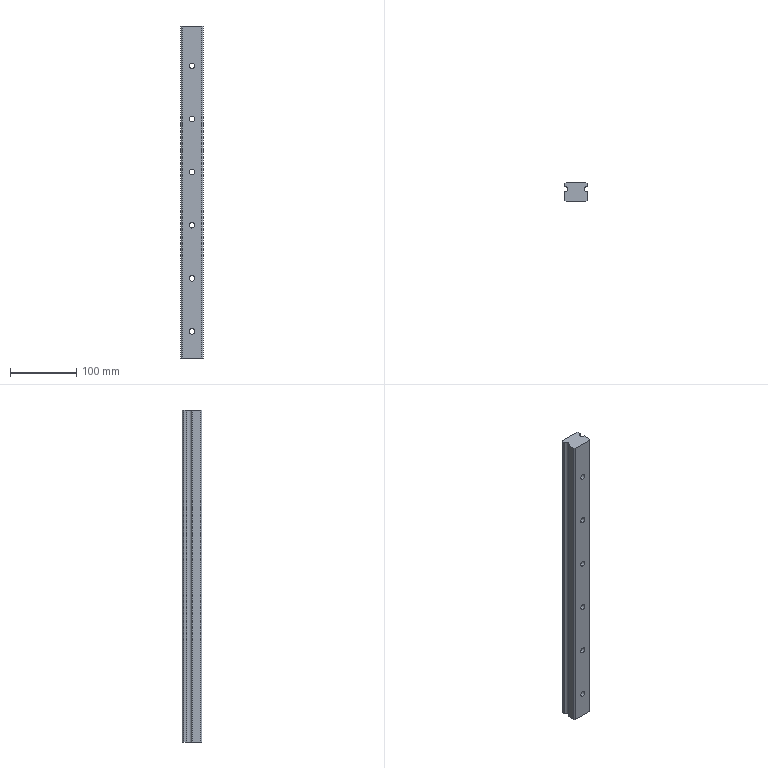Part | Creo | features CUT 7, CURVE 3, DATUM PLANE 3, COORDINATE SYSTEM 1, PATTERN 1, PROTRUSION 1 | 1 solid | 44 faces | box 33.99 x 29 x 500 mm | volume 443618 mm3 | cylinder 26 | plane 18 | commonest cylinder face diameters 8.5 x12 14 x12 8.76 x2
STEP:
#1=CARTESIAN_POINT('',(0.,0.,0.));
#2=DIRECTION('',(0.,0.,1.));
#3=DIRECTION('',(1.,0.,0.));
#4=AXIS2_PLACEMENT_3D('',#1,#2,#3);
#5=CARTESIAN_POINT('',(-14.995,0.,-250.));
#6=VERTEX_POINT('',#5);
#7=CARTESIAN_POINT('',(15.005,0.,-250.));
#8=VERTEX_POINT('',#7);
#9=CARTESIAN_POINT('',(-14.995,0.,-250.));
#10=DIRECTION('',(1.,0.,0.));
#11=VECTOR('',#10,30.);
#12=LINE('',#9,#11);
#13=EDGE_CURVE('',#6,#8,#12,.T.);
#14=ORIENTED_EDGE('',*,*,#13,.T.);
#15=CARTESIAN_POINT('',(17.,1.995,-250.));
#16=VERTEX_POINT('',#15);
#17=CARTESIAN_POINT('',(15.005,0.,-250.));
#18=DIRECTION('',(0.7071,0.7071,0.));
#19=VECTOR('',#18,2.821);
#20=LINE('',#17,#19);
#21=EDGE_CURVE('',#8,#16,#20,.T.);
#22=ORIENTED_EDGE('',*,*,#21,.T.);
#23=CARTESIAN_POINT('',(17.,14.215,-250.));
#24=VERTEX_POINT('',#23);
#25=CARTESIAN_POINT('',(17.,1.995,-250.));
#26=DIRECTION('',(0.,1.,0.));
#27=VECTOR('',#26,12.22);
#28=LINE('',#25,#27);
#29=EDGE_CURVE('',#16,#24,#28,.T.);
#30=ORIENTED_EDGE('',*,*,#29,.T.);
#31=CARTESIAN_POINT('',(17.,22.975,-250.));
#32=VERTEX_POINT('',#31);
#33=CARTESIAN_POINT('',(17.,18.595,-250.));
#34=DIRECTION('',(0.,0.,-1.));
#35=DIRECTION('',(0.,-1.,0.));
#36=AXIS2_PLACEMENT_3D('',#33,#34,#35);
#37=CIRCLE('',#36,4.38);
#38=EDGE_CURVE('',#24,#32,#37,.T.);
#39=ORIENTED_EDGE('',*,*,#38,.T.);
#40=CARTESIAN_POINT('',(17.,27.005,-250.));
#41=VERTEX_POINT('',#40);
#42=CARTESIAN_POINT('',(17.,22.975,-250.));
#43=DIRECTION('',(0.,1.,0.));
#44=VECTOR('',#43,4.03);
#45=LINE('',#42,#44);
#46=EDGE_CURVE('',#32,#41,#45,.T.);
#47=ORIENTED_EDGE('',*,*,#46,.T.);
#48=CARTESIAN_POINT('',(15.005,29.,-250.));
#49=VERTEX_POINT('',#48);
#50=CARTESIAN_POINT('',(17.,27.005,-250.));
#51=DIRECTION('',(-0.7071,0.7071,0.));
#52=VECTOR('',#51,2.821);
#53=LINE('',#50,#52);
#54=EDGE_CURVE('',#41,#49,#53,.T.);
#55=ORIENTED_EDGE('',*,*,#54,.T.);
#56=CARTESIAN_POINT('',(-14.995,29.,-250.));
#57=VERTEX_POINT('',#56);
#58=CARTESIAN_POINT('',(15.005,29.,-250.));
#59=DIRECTION('',(-1.,0.,0.));
#60=VECTOR('',#59,30.);
#61=LINE('',#58,#60);
#62=EDGE_CURVE('',#49,#57,#61,.T.);
#63=ORIENTED_EDGE('',*,*,#62,.T.);
#64=CARTESIAN_POINT('',(-16.99,27.005,-250.));
#65=VERTEX_POINT('',#64);
#66=CARTESIAN_POINT('',(-14.995,29.,-250.));
#67=DIRECTION('',(-0.7071,-0.7071,0.));
#68=VECTOR('',#67,2.821);
#69=LINE('',#66,#68);
#70=EDGE_CURVE('',#57,#65,#69,.T.);
#71=ORIENTED_EDGE('',*,*,#70,.T.);
#72=CARTESIAN_POINT('',(-16.99,22.975,-250.));
#73=VERTEX_POINT('',#72);
#74=CARTESIAN_POINT('',(-16.99,27.005,-250.));
#75=DIRECTION('',(0.,-1.,0.));
#76=VECTOR('',#75,4.03);
#77=LINE('',#74,#76);
#78=EDGE_CURVE('',#65,#73,#77,.T.);
#79=ORIENTED_EDGE('',*,*,#78,.T.);
#80=CARTESIAN_POINT('',(-16.99,14.215,-250.));
#81=VERTEX_POINT('',#80);
#82=CARTESIAN_POINT('',(-16.99,18.595,-250.));
#83=DIRECTION('',(0.,0.,-1.));
#84=DIRECTION('',(0.,1.,0.));
#85=AXIS2_PLACEMENT_3D('',#82,#83,#84);
#86=CIRCLE('',#85,4.38);
#87=EDGE_CURVE('',#73,#81,#86,.T.);
#88=ORIENTED_EDGE('',*,*,#87,.T.);
#89=CARTESIAN_POINT('',(-16.99,1.995,-250.));
#90=VERTEX_POINT('',#89);
#91=CARTESIAN_POINT('',(-16.99,14.215,-250.));
#92=DIRECTION('',(0.,-1.,0.));
#93=VECTOR('',#92,12.22);
#94=LINE('',#91,#93);
#95=EDGE_CURVE('',#81,#90,#94,.T.);
#96=ORIENTED_EDGE('',*,*,#95,.T.);
#97=CARTESIAN_POINT('',(-16.99,1.995,-250.));
#98=DIRECTION('',(0.7071,-0.7071,0.));
#99=VECTOR('',#98,2.821);
#100=LINE('',#97,#99);
#101=EDGE_CURVE('',#90,#6,#100,.T.);
#102=ORIENTED_EDGE('',*,*,#101,.T.);
#103=EDGE_LOOP('',(#14,#22,#30,#39,#47,#55,#63,#71,#79,#88,#96,#102));
#104=FACE_OUTER_BOUND('',#103,.F.);
#105=CARTESIAN_POINT('',(0.,0.,-250.));
#106=DIRECTION('',(0.,0.,1.));
#107=DIRECTION('',(1.,0.,0.));
#108=AXIS2_PLACEMENT_3D('',#105,#106,#107);
#109=PLANE('',#108);
#110=ADVANCED_FACE('',(#104),#109,.F.);
#111=ORIENTED_EDGE('',*,*,#13,.F.);
#112=CARTESIAN_POINT('',(-14.995,0.,250.));
#113=VERTEX_POINT('',#112);
#114=CARTESIAN_POINT('',(-14.995,0.,-250.));
#115=DIRECTION('',(0.,0.,1.));
#116=VECTOR('',#115,500.);
#117=LINE('',#114,#116);
#118=EDGE_CURVE('',#6,#113,#117,.T.);
#119=ORIENTED_EDGE('',*,*,#118,.T.);
#120=CARTESIAN_POINT('',(15.005,0.,250.));
#121=VERTEX_POINT('',#120);
#122=CARTESIAN_POINT('',(-14.995,0.,250.));
#123=DIRECTION('',(1.,0.,0.));
#124=VECTOR('',#123,30.);
#125=LINE('',#122,#124);
#126=EDGE_CURVE('',#113,#121,#125,.T.);
#127=ORIENTED_EDGE('',*,*,#126,.T.);
#128=CARTESIAN_POINT('',(15.005,0.,-250.));
#129=DIRECTION('',(0.,0.,1.));
#130=VECTOR('',#129,500.);
#131=LINE('',#128,#130);
#132=EDGE_CURVE('',#8,#121,#131,.T.);
#133=ORIENTED_EDGE('',*,*,#132,.F.);
#134=EDGE_LOOP('',(#111,#119,#127,#133));
#135=FACE_OUTER_BOUND('',#134,.F.);
#136=CARTESIAN_POINT('',(0.,0.,-214.25));
#137=VERTEX_POINT('',#136);
#138=CARTESIAN_POINT('',(0.,0.,-205.75));
#139=VERTEX_POINT('',#138);
#140=CARTESIAN_POINT('',(0.,0.,-210.));
#141=DIRECTION('',(0.,1.,0.));
#142=DIRECTION('',(0.,0.,-1.));
#143=AXIS2_PLACEMENT_3D('',#140,#141,#142);
#144=CIRCLE('',#143,4.25);
#145=EDGE_CURVE('',#137,#139,#144,.T.);
#146=ORIENTED_EDGE('',*,*,#145,.F.);
#147=CARTESIAN_POINT('',(0.,0.,-210.));
#148=DIRECTION('',(0.,1.,0.));
#149=DIRECTION('',(0.,0.,1.));
#150=AXIS2_PLACEMENT_3D('',#147,#148,#149);
#151=CIRCLE('',#150,4.25);
#152=EDGE_CURVE('',#139,#137,#151,.T.);
#153=ORIENTED_EDGE('',*,*,#152,.F.);
#154=EDGE_LOOP('',(#146,#153));
#155=FACE_BOUND('',#154,.F.);
#156=CARTESIAN_POINT('',(0.,0.,-134.25));
#157=VERTEX_POINT('',#156);
#158=CARTESIAN_POINT('',(0.,0.,-125.75));
#159=VERTEX_POINT('',#158);
#160=CARTESIAN_POINT('',(0.,0.,-130.));
#161=DIRECTION('',(0.,1.,0.));
#162=DIRECTION('',(0.,0.,-1.));
#163=AXIS2_PLACEMENT_3D('',#160,#161,#162);
#164=CIRCLE('',#163,4.25);
#165=EDGE_CURVE('',#157,#159,#164,.T.);
#166=ORIENTED_EDGE('',*,*,#165,.F.);
#167=CARTESIAN_POINT('',(0.,0.,-130.));
#168=DIRECTION('',(0.,1.,0.));
#169=DIRECTION('',(0.,0.,1.));
#170=AXIS2_PLACEMENT_3D('',#167,#168,#169);
#171=CIRCLE('',#170,4.25);
#172=EDGE_CURVE('',#159,#157,#171,.T.);
#173=ORIENTED_EDGE('',*,*,#172,.F.);
#174=EDGE_LOOP('',(#166,#173));
#175=FACE_BOUND('',#174,.F.);
#176=CARTESIAN_POINT('',(0.,0.,-54.25));
#177=VERTEX_POINT('',#176);
#178=CARTESIAN_POINT('',(0.,0.,-45.75));
#179=VERTEX_POINT('',#178);
#180=CARTESIAN_POINT('',(0.,0.,-50.));
#181=DIRECTION('',(0.,1.,0.));
#182=DIRECTION('',(0.,0.,-1.));
#183=AXIS2_PLACEMENT_3D('',#180,#181,#182);
#184=CIRCLE('',#183,4.25);
#185=EDGE_CURVE('',#177,#179,#184,.T.);
#186=ORIENTED_EDGE('',*,*,#185,.F.);
#187=CARTESIAN_POINT('',(0.,0.,-50.));
#188=DIRECTION('',(0.,1.,0.));
#189=DIRECTION('',(0.,0.,1.));
#190=AXIS2_PLACEMENT_3D('',#187,#188,#189);
#191=CIRCLE('',#190,4.25);
#192=EDGE_CURVE('',#179,#177,#191,.T.);
#193=ORIENTED_EDGE('',*,*,#192,.F.);
#194=EDGE_LOOP('',(#186,#193));
#195=FACE_BOUND('',#194,.F.);
#196=CARTESIAN_POINT('',(0.,0.,25.75));
#197=VERTEX_POINT('',#196);
#198=CARTESIAN_POINT('',(0.,0.,34.25));
#199=VERTEX_POINT('',#198);
#200=CARTESIAN_POINT('',(0.,0.,30.));
#201=DIRECTION('',(0.,1.,0.));
#202=DIRECTION('',(0.,0.,-1.));
#203=AXIS2_PLACEMENT_3D('',#200,#201,#202);
#204=CIRCLE('',#203,4.25);
#205=EDGE_CURVE('',#197,#199,#204,.T.);
#206=ORIENTED_EDGE('',*,*,#205,.F.);
#207=CARTESIAN_POINT('',(0.,0.,30.));
#208=DIRECTION('',(0.,1.,0.));
#209=DIRECTION('',(0.,0.,1.));
#210=AXIS2_PLACEMENT_3D('',#207,#208,#209);
#211=CIRCLE('',#210,4.25);
#212=EDGE_CURVE('',#199,#197,#211,.T.);
#213=ORIENTED_EDGE('',*,*,#212,.F.);
#214=EDGE_LOOP('',(#206,#213));
#215=FACE_BOUND('',#214,.F.);
#216=CARTESIAN_POINT('',(0.,0.,105.75));
#217=VERTEX_POINT('',#216);
#218=CARTESIAN_POINT('',(0.,0.,114.25));
#219=VERTEX_POINT('',#218);
#220=CARTESIAN_POINT('',(0.,0.,110.));
#221=DIRECTION('',(0.,1.,0.));
#222=DIRECTION('',(0.,0.,-1.));
#223=AXIS2_PLACEMENT_3D('',#220,#221,#222);
#224=CIRCLE('',#223,4.25);
#225=EDGE_CURVE('',#217,#219,#224,.T.);
#226=ORIENTED_EDGE('',*,*,#225,.F.);
#227=CARTESIAN_POINT('',(0.,0.,110.));
#228=DIRECTION('',(0.,1.,0.));
#229=DIRECTION('',(0.,0.,1.));
#230=AXIS2_PLACEMENT_3D('',#227,#228,#229);
#231=CIRCLE('',#230,4.25);
#232=EDGE_CURVE('',#219,#217,#231,.T.);
#233=ORIENTED_EDGE('',*,*,#232,.F.);
#234=EDGE_LOOP('',(#226,#233));
#235=FACE_BOUND('',#234,.F.);
#236=CARTESIAN_POINT('',(0.,0.,185.75));
#237=VERTEX_POINT('',#236);
#238=CARTESIAN_POINT('',(0.,0.,194.25));
#239=VERTEX_POINT('',#238);
#240=CARTESIAN_POINT('',(0.,0.,190.));
#241=DIRECTION('',(0.,1.,0.));
#242=DIRECTION('',(0.,0.,-1.));
#243=AXIS2_PLACEMENT_3D('',#240,#241,#242);
#244=CIRCLE('',#243,4.25);
#245=EDGE_CURVE('',#237,#239,#244,.T.);
#246=ORIENTED_EDGE('',*,*,#245,.F.);
#247=CARTESIAN_POINT('',(0.,0.,190.));
#248=DIRECTION('',(0.,1.,0.));
#249=DIRECTION('',(0.,0.,1.));
#250=AXIS2_PLACEMENT_3D('',#247,#248,#249);
#251=CIRCLE('',#250,4.25);
#252=EDGE_CURVE('',#239,#237,#251,.T.);
#253=ORIENTED_EDGE('',*,*,#252,.F.);
#254=EDGE_LOOP('',(#246,#253));
#255=FACE_BOUND('',#254,.F.);
#256=CARTESIAN_POINT('',(-14.995,0.,-250.));
#257=DIRECTION('',(0.,-1.,0.));
#258=DIRECTION('',(1.,0.,0.));
#259=AXIS2_PLACEMENT_3D('',#256,#257,#258);
#260=PLANE('',#259);
#261=ADVANCED_FACE('',(#135,#155,#175,#195,#215,#235,#255),#260,.T.);
#262=ORIENTED_EDGE('',*,*,#101,.F.);
#263=CARTESIAN_POINT('',(-16.99,1.995,250.));
#264=VERTEX_POINT('',#263);
#265=CARTESIAN_POINT('',(-16.99,1.995,-250.));
#266=DIRECTION('',(0.,0.,1.));
#267=VECTOR('',#266,500.);
#268=LINE('',#265,#267);
#269=EDGE_CURVE('',#90,#264,#268,.T.);
#270=ORIENTED_EDGE('',*,*,#269,.T.);
#271=CARTESIAN_POINT('',(-16.99,1.995,250.));
#272=DIRECTION('',(0.7071,-0.7071,0.));
#273=VECTOR('',#272,2.821);
#274=LINE('',#271,#273);
#275=EDGE_CURVE('',#264,#113,#274,.T.);
#276=ORIENTED_EDGE('',*,*,#275,.T.);
#277=ORIENTED_EDGE('',*,*,#118,.F.);
#278=EDGE_LOOP('',(#262,#270,#276,#277));
#279=FACE_OUTER_BOUND('',#278,.F.);
#280=CARTESIAN_POINT('',(-16.99,1.995,-250.));
#281=DIRECTION('',(-0.7071,-0.7071,0.));
#282=DIRECTION('',(0.7071,-0.7071,0.));
#283=AXIS2_PLACEMENT_3D('',#280,#281,#282);
#284=PLANE('',#283);
#285=ADVANCED_FACE('',(#279),#284,.T.);
#286=ORIENTED_EDGE('',*,*,#95,.F.);
#287=CARTESIAN_POINT('',(-16.99,14.215,250.));
#288=VERTEX_POINT('',#287);
#289=CARTESIAN_POINT('',(-16.99,14.215,-250.));
#290=DIRECTION('',(0.,0.,1.));
#291=VECTOR('',#290,500.);
#292=LINE('',#289,#291);
#293=EDGE_CURVE('',#81,#288,#292,.T.);
#294=ORIENTED_EDGE('',*,*,#293,.T.);
#295=CARTESIAN_POINT('',(-16.99,14.215,250.));
#296=DIRECTION('',(0.,-1.,0.));
#297=VECTOR('',#296,12.22);
#298=LINE('',#295,#297);
#299=EDGE_CURVE('',#288,#264,#298,.T.);
#300=ORIENTED_EDGE('',*,*,#299,.T.);
#301=ORIENTED_EDGE('',*,*,#269,.F.);
#302=EDGE_LOOP('',(#286,#294,#300,#301));
#303=FACE_OUTER_BOUND('',#302,.F.);
#304=CARTESIAN_POINT('',(-16.99,14.215,-250.));
#305=DIRECTION('',(-1.,0.,0.));
#306=DIRECTION('',(0.,-1.,0.));
#307=AXIS2_PLACEMENT_3D('',#304,#305,#306);
#308=PLANE('',#307);
#309=ADVANCED_FACE('',(#303),#308,.T.);
#310=ORIENTED_EDGE('',*,*,#87,.F.);
#311=CARTESIAN_POINT('',(-16.99,22.975,250.));
#312=VERTEX_POINT('',#311);
#313=CARTESIAN_POINT('',(-16.99,22.975,-250.));
#314=DIRECTION('',(0.,0.,1.));
#315=VECTOR('',#314,500.);
#316=LINE('',#313,#315);
#317=EDGE_CURVE('',#73,#312,#316,.T.);
#318=ORIENTED_EDGE('',*,*,#317,.T.);
#319=CARTESIAN_POINT('',(-16.99,18.595,250.));
#320=DIRECTION('',(0.,0.,-1.));
#321=DIRECTION('',(0.,1.,0.));
#322=AXIS2_PLACEMENT_3D('',#319,#320,#321);
#323=CIRCLE('',#322,4.38);
#324=EDGE_CURVE('',#312,#288,#323,.T.);
#325=ORIENTED_EDGE('',*,*,#324,.T.);
#326=ORIENTED_EDGE('',*,*,#293,.F.);
#327=EDGE_LOOP('',(#310,#318,#325,#326));
#328=FACE_OUTER_BOUND('',#327,.F.);
#329=CARTESIAN_POINT('',(-16.99,18.595,-250.));
#330=DIRECTION('',(0.,0.,1.));
#331=DIRECTION('',(1.,0.,0.));
#332=AXIS2_PLACEMENT_3D('',#329,#330,#331);
#333=CYLINDRICAL_SURFACE('',#332,4.38);
#334=ADVANCED_FACE('',(#328),#333,.F.);
#335=ORIENTED_EDGE('',*,*,#78,.F.);
#336=CARTESIAN_POINT('',(-16.99,27.005,250.));
#337=VERTEX_POINT('',#336);
#338=CARTESIAN_POINT('',(-16.99,27.005,-250.));
#339=DIRECTION('',(0.,0.,1.));
#340=VECTOR('',#339,500.);
#341=LINE('',#338,#340);
#342=EDGE_CURVE('',#65,#337,#341,.T.);
#343=ORIENTED_EDGE('',*,*,#342,.T.);
#344=CARTESIAN_POINT('',(-16.99,27.005,250.));
#345=DIRECTION('',(0.,-1.,0.));
#346=VECTOR('',#345,4.03);
#347=LINE('',#344,#346);
#348=EDGE_CURVE('',#337,#312,#347,.T.);
#349=ORIENTED_EDGE('',*,*,#348,.T.);
#350=ORIENTED_EDGE('',*,*,#317,.F.);
#351=EDGE_LOOP('',(#335,#343,#349,#350));
#352=FACE_OUTER_BOUND('',#351,.F.);
#353=CARTESIAN_POINT('',(-16.99,27.005,-250.));
#354=DIRECTION('',(-1.,0.,0.));
#355=DIRECTION('',(0.,-1.,0.));
#356=AXIS2_PLACEMENT_3D('',#353,#354,#355);
#357=PLANE('',#356);
#358=ADVANCED_FACE('',(#352),#357,.T.);
#359=ORIENTED_EDGE('',*,*,#70,.F.);
#360=CARTESIAN_POINT('',(-14.995,29.,250.));
#361=VERTEX_POINT('',#360);
#362=CARTESIAN_POINT('',(-14.995,29.,-250.));
#363=DIRECTION('',(0.,0.,1.));
#364=VECTOR('',#363,500.);
#365=LINE('',#362,#364);
#366=EDGE_CURVE('',#57,#361,#365,.T.);
#367=ORIENTED_EDGE('',*,*,#366,.T.);
#368=CARTESIAN_POINT('',(-14.995,29.,250.));
#369=DIRECTION('',(-0.7071,-0.7071,0.));
#370=VECTOR('',#369,2.821);
#371=LINE('',#368,#370);
#372=EDGE_CURVE('',#361,#337,#371,.T.);
#373=ORIENTED_EDGE('',*,*,#372,.T.);
#374=ORIENTED_EDGE('',*,*,#342,.F.);
#375=EDGE_LOOP('',(#359,#367,#373,#374));
#376=FACE_OUTER_BOUND('',#375,.F.);
#377=CARTESIAN_POINT('',(-14.995,29.,-250.));
#378=DIRECTION('',(-0.7071,0.7071,0.));
#379=DIRECTION('',(-0.7071,-0.7071,0.));
#380=AXIS2_PLACEMENT_3D('',#377,#378,#379);
#381=PLANE('',#380);
#382=ADVANCED_FACE('',(#376),#381,.T.);
#383=ORIENTED_EDGE('',*,*,#62,.F.);
#384=CARTESIAN_POINT('',(15.005,29.,250.));
#385=VERTEX_POINT('',#384);
#386=CARTESIAN_POINT('',(15.005,29.,-250.));
#387=DIRECTION('',(0.,0.,1.));
#388=VECTOR('',#387,500.);
#389=LINE('',#386,#388);
#390=EDGE_CURVE('',#49,#385,#389,.T.);
#391=ORIENTED_EDGE('',*,*,#390,.T.);
#392=CARTESIAN_POINT('',(15.005,29.,250.));
#393=DIRECTION('',(-1.,0.,0.));
#394=VECTOR('',#393,30.);
#395=LINE('',#392,#394);
#396=EDGE_CURVE('',#385,#361,#395,.T.);
#397=ORIENTED_EDGE('',*,*,#396,.T.);
#398=ORIENTED_EDGE('',*,*,#366,.F.);
#399=EDGE_LOOP('',(#383,#391,#397,#398));
#400=FACE_OUTER_BOUND('',#399,.F.);
#401=CARTESIAN_POINT('',(0.,29.,-217.));
#402=VERTEX_POINT('',#401);
#403=CARTESIAN_POINT('',(0.,29.,-203.));
#404=VERTEX_POINT('',#403);
#405=CARTESIAN_POINT('',(0.,29.,-210.));
#406=DIRECTION('',(0.,1.,0.));
#407=DIRECTION('',(0.,0.,-1.));
#408=AXIS2_PLACEMENT_3D('',#405,#406,#407);
#409=CIRCLE('',#408,7.);
#410=EDGE_CURVE('',#402,#404,#409,.T.);
#411=ORIENTED_EDGE('',*,*,#410,.T.);
#412=CARTESIAN_POINT('',(0.,29.,-210.));
#413=DIRECTION('',(0.,1.,0.));
#414=DIRECTION('',(0.,0.,1.));
#415=AXIS2_PLACEMENT_3D('',#412,#413,#414);
#416=CIRCLE('',#415,7.);
#417=EDGE_CURVE('',#404,#402,#416,.T.);
#418=ORIENTED_EDGE('',*,*,#417,.T.);
#419=EDGE_LOOP('',(#411,#418));
#420=FACE_BOUND('',#419,.F.);
#421=CARTESIAN_POINT('',(0.,29.,-137.));
#422=VERTEX_POINT('',#421);
#423=CARTESIAN_POINT('',(0.,29.,-123.));
#424=VERTEX_POINT('',#423);
#425=CARTESIAN_POINT('',(0.,29.,-130.));
#426=DIRECTION('',(0.,1.,0.));
#427=DIRECTION('',(0.,0.,-1.));
#428=AXIS2_PLACEMENT_3D('',#425,#426,#427);
#429=CIRCLE('',#428,7.);
#430=EDGE_CURVE('',#422,#424,#429,.T.);
#431=ORIENTED_EDGE('',*,*,#430,.T.);
#432=CARTESIAN_POINT('',(0.,29.,-130.));
#433=DIRECTION('',(0.,1.,0.));
#434=DIRECTION('',(0.,0.,1.));
#435=AXIS2_PLACEMENT_3D('',#432,#433,#434);
#436=CIRCLE('',#435,7.);
#437=EDGE_CURVE('',#424,#422,#436,.T.);
#438=ORIENTED_EDGE('',*,*,#437,.T.);
#439=EDGE_LOOP('',(#431,#438));
#440=FACE_BOUND('',#439,.F.);
#441=CARTESIAN_POINT('',(0.,29.,-57.));
#442=VERTEX_POINT('',#441);
#443=CARTESIAN_POINT('',(0.,29.,-43.));
#444=VERTEX_POINT('',#443);
#445=CARTESIAN_POINT('',(0.,29.,-50.));
#446=DIRECTION('',(0.,1.,0.));
#447=DIRECTION('',(0.,0.,-1.));
#448=AXIS2_PLACEMENT_3D('',#445,#446,#447);
#449=CIRCLE('',#448,7.);
#450=EDGE_CURVE('',#442,#444,#449,.T.);
#451=ORIENTED_EDGE('',*,*,#450,.T.);
#452=CARTESIAN_POINT('',(0.,29.,-50.));
#453=DIRECTION('',(0.,1.,0.));
#454=DIRECTION('',(0.,0.,1.));
#455=AXIS2_PLACEMENT_3D('',#452,#453,#454);
#456=CIRCLE('',#455,7.);
#457=EDGE_CURVE('',#444,#442,#456,.T.);
#458=ORIENTED_EDGE('',*,*,#457,.T.);
#459=EDGE_LOOP('',(#451,#458));
#460=FACE_BOUND('',#459,.F.);
#461=CARTESIAN_POINT('',(0.,29.,23.));
#462=VERTEX_POINT('',#461);
#463=CARTESIAN_POINT('',(0.,29.,37.));
#464=VERTEX_POINT('',#463);
#465=CARTESIAN_POINT('',(0.,29.,30.));
#466=DIRECTION('',(0.,1.,0.));
#467=DIRECTION('',(0.,0.,-1.));
#468=AXIS2_PLACEMENT_3D('',#465,#466,#467);
#469=CIRCLE('',#468,7.);
#470=EDGE_CURVE('',#462,#464,#469,.T.);
#471=ORIENTED_EDGE('',*,*,#470,.T.);
#472=CARTESIAN_POINT('',(0.,29.,30.));
#473=DIRECTION('',(0.,1.,0.));
#474=DIRECTION('',(0.,0.,1.));
#475=AXIS2_PLACEMENT_3D('',#472,#473,#474);
#476=CIRCLE('',#475,7.);
#477=EDGE_CURVE('',#464,#462,#476,.T.);
#478=ORIENTED_EDGE('',*,*,#477,.T.);
#479=EDGE_LOOP('',(#471,#478));
#480=FACE_BOUND('',#479,.F.);
#481=CARTESIAN_POINT('',(0.,29.,103.));
#482=VERTEX_POINT('',#481);
#483=CARTESIAN_POINT('',(0.,29.,117.));
#484=VERTEX_POINT('',#483);
#485=CARTESIAN_POINT('',(0.,29.,110.));
#486=DIRECTION('',(0.,1.,0.));
#487=DIRECTION('',(0.,0.,-1.));
#488=AXIS2_PLACEMENT_3D('',#485,#486,#487);
#489=CIRCLE('',#488,7.);
#490=EDGE_CURVE('',#482,#484,#489,.T.);
#491=ORIENTED_EDGE('',*,*,#490,.T.);
#492=CARTESIAN_POINT('',(0.,29.,110.));
#493=DIRECTION('',(0.,1.,0.));
#494=DIRECTION('',(0.,0.,1.));
#495=AXIS2_PLACEMENT_3D('',#492,#493,#494);
#496=CIRCLE('',#495,7.);
#497=EDGE_CURVE('',#484,#482,#496,.T.);
#498=ORIENTED_EDGE('',*,*,#497,.T.);
#499=EDGE_LOOP('',(#491,#498));
#500=FACE_BOUND('',#499,.F.);
#501=CARTESIAN_POINT('',(0.,29.,183.));
#502=VERTEX_POINT('',#501);
#503=CARTESIAN_POINT('',(0.,29.,197.));
#504=VERTEX_POINT('',#503);
#505=CARTESIAN_POINT('',(0.,29.,190.));
#506=DIRECTION('',(0.,1.,0.));
#507=DIRECTION('',(0.,0.,-1.));
#508=AXIS2_PLACEMENT_3D('',#505,#506,#507);
#509=CIRCLE('',#508,7.);
#510=EDGE_CURVE('',#502,#504,#509,.T.);
#511=ORIENTED_EDGE('',*,*,#510,.T.);
#512=CARTESIAN_POINT('',(0.,29.,190.));
#513=DIRECTION('',(0.,1.,0.));
#514=DIRECTION('',(0.,0.,1.));
#515=AXIS2_PLACEMENT_3D('',#512,#513,#514);
#516=CIRCLE('',#515,7.);
#517=EDGE_CURVE('',#504,#502,#516,.T.);
#518=ORIENTED_EDGE('',*,*,#517,.T.);
#519=EDGE_LOOP('',(#511,#518));
#520=FACE_BOUND('',#519,.F.);
#521=CARTESIAN_POINT('',(15.005,29.,-250.));
#522=DIRECTION('',(0.,1.,0.));
#523=DIRECTION('',(-1.,0.,0.));
#524=AXIS2_PLACEMENT_3D('',#521,#522,#523);
#525=PLANE('',#524);
#526=ADVANCED_FACE('',(#400,#420,#440,#460,#480,#500,#520),#525,.T.);
#527=ORIENTED_EDGE('',*,*,#54,.F.);
#528=CARTESIAN_POINT('',(17.,27.005,250.));
#529=VERTEX_POINT('',#528);
#530=CARTESIAN_POINT('',(17.,27.005,-250.));
#531=DIRECTION('',(0.,0.,1.));
#532=VECTOR('',#531,500.);
#533=LINE('',#530,#532);
#534=EDGE_CURVE('',#41,#529,#533,.T.);
#535=ORIENTED_EDGE('',*,*,#534,.T.);
#536=CARTESIAN_POINT('',(17.,27.005,250.));
#537=DIRECTION('',(-0.7071,0.7071,0.));
#538=VECTOR('',#537,2.821);
#539=LINE('',#536,#538);
#540=EDGE_CURVE('',#529,#385,#539,.T.);
#541=ORIENTED_EDGE('',*,*,#540,.T.);
#542=ORIENTED_EDGE('',*,*,#390,.F.);
#543=EDGE_LOOP('',(#527,#535,#541,#542));
#544=FACE_OUTER_BOUND('',#543,.F.);
#545=CARTESIAN_POINT('',(17.,27.005,-250.));
#546=DIRECTION('',(0.7071,0.7071,0.));
#547=DIRECTION('',(-0.7071,0.7071,0.));
#548=AXIS2_PLACEMENT_3D('',#545,#546,#547);
#549=PLANE('',#548);
#550=ADVANCED_FACE('',(#544),#549,.T.);
#551=ORIENTED_EDGE('',*,*,#46,.F.);
#552=CARTESIAN_POINT('',(17.,22.975,250.));
#553=VERTEX_POINT('',#552);
#554=CARTESIAN_POINT('',(17.,22.975,-250.));
#555=DIRECTION('',(0.,0.,1.));
#556=VECTOR('',#555,500.);
#557=LINE('',#554,#556);
#558=EDGE_CURVE('',#32,#553,#557,.T.);
#559=ORIENTED_EDGE('',*,*,#558,.T.);
#560=CARTESIAN_POINT('',(17.,22.975,250.));
#561=DIRECTION('',(0.,1.,0.));
#562=VECTOR('',#561,4.03);
#563=LINE('',#560,#562);
#564=EDGE_CURVE('',#553,#529,#563,.T.);
#565=ORIENTED_EDGE('',*,*,#564,.T.);
#566=ORIENTED_EDGE('',*,*,#534,.F.);
#567=EDGE_LOOP('',(#551,#559,#565,#566));
#568=FACE_OUTER_BOUND('',#567,.F.);
#569=CARTESIAN_POINT('',(17.,22.975,-250.));
#570=DIRECTION('',(1.,0.,0.));
#571=DIRECTION('',(0.,1.,0.));
#572=AXIS2_PLACEMENT_3D('',#569,#570,#571);
#573=PLANE('',#572);
#574=ADVANCED_FACE('',(#568),#573,.T.);
#575=ORIENTED_EDGE('',*,*,#38,.F.);
#576=CARTESIAN_POINT('',(17.,14.215,250.));
#577=VERTEX_POINT('',#576);
#578=CARTESIAN_POINT('',(17.,14.215,-250.));
#579=DIRECTION('',(0.,0.,1.));
#580=VECTOR('',#579,500.);
#581=LINE('',#578,#580);
#582=EDGE_CURVE('',#24,#577,#581,.T.);
#583=ORIENTED_EDGE('',*,*,#582,.T.);
#584=CARTESIAN_POINT('',(17.,18.595,250.));
#585=DIRECTION('',(0.,0.,-1.));
#586=DIRECTION('',(0.,-1.,0.));
#587=AXIS2_PLACEMENT_3D('',#584,#585,#586);
#588=CIRCLE('',#587,4.38);
#589=EDGE_CURVE('',#577,#553,#588,.T.);
#590=ORIENTED_EDGE('',*,*,#589,.T.);
#591=ORIENTED_EDGE('',*,*,#558,.F.);
#592=EDGE_LOOP('',(#575,#583,#590,#591));
#593=FACE_OUTER_BOUND('',#592,.F.);
#594=CARTESIAN_POINT('',(17.,18.595,-250.));
#595=DIRECTION('',(0.,0.,1.));
#596=DIRECTION('',(1.,0.,0.));
#597=AXIS2_PLACEMENT_3D('',#594,#595,#596);
#598=CYLINDRICAL_SURFACE('',#597,4.38);
#599=ADVANCED_FACE('',(#593),#598,.F.);
#600=ORIENTED_EDGE('',*,*,#29,.F.);
#601=CARTESIAN_POINT('',(17.,1.995,250.));
#602=VERTEX_POINT('',#601);
#603=CARTESIAN_POINT('',(17.,1.995,-250.));
#604=DIRECTION('',(0.,0.,1.));
#605=VECTOR('',#604,500.);
#606=LINE('',#603,#605);
#607=EDGE_CURVE('',#16,#602,#606,.T.);
#608=ORIENTED_EDGE('',*,*,#607,.T.);
#609=CARTESIAN_POINT('',(17.,1.995,250.));
#610=DIRECTION('',(0.,1.,0.));
#611=VECTOR('',#610,12.22);
#612=LINE('',#609,#611);
#613=EDGE_CURVE('',#602,#577,#612,.T.);
#614=ORIENTED_EDGE('',*,*,#613,.T.);
#615=ORIENTED_EDGE('',*,*,#582,.F.);
#616=EDGE_LOOP('',(#600,#608,#614,#615));
#617=FACE_OUTER_BOUND('',#616,.F.);
#618=CARTESIAN_POINT('',(17.,1.995,-250.));
#619=DIRECTION('',(1.,0.,0.));
#620=DIRECTION('',(0.,1.,0.));
#621=AXIS2_PLACEMENT_3D('',#618,#619,#620);
#622=PLANE('',#621);
#623=ADVANCED_FACE('',(#617),#622,.T.);
#624=ORIENTED_EDGE('',*,*,#21,.F.);
#625=ORIENTED_EDGE('',*,*,#132,.T.);
#626=CARTESIAN_POINT('',(15.005,0.,250.));
#627=DIRECTION('',(0.7071,0.7071,0.));
#628=VECTOR('',#627,2.821);
#629=LINE('',#626,#628);
#630=EDGE_CURVE('',#121,#602,#629,.T.);
#631=ORIENTED_EDGE('',*,*,#630,.T.);
#632=ORIENTED_EDGE('',*,*,#607,.F.);
#633=EDGE_LOOP('',(#624,#625,#631,#632));
#634=FACE_OUTER_BOUND('',#633,.F.);
#635=CARTESIAN_POINT('',(15.005,0.,-250.));
#636=DIRECTION('',(0.7071,-0.7071,0.));
#637=DIRECTION('',(0.7071,0.7071,0.));
#638=AXIS2_PLACEMENT_3D('',#635,#636,#637);
#639=PLANE('',#638);
#640=ADVANCED_FACE('',(#634),#639,.T.);
#641=ORIENTED_EDGE('',*,*,#126,.F.);
#642=ORIENTED_EDGE('',*,*,#275,.F.);
#643=ORIENTED_EDGE('',*,*,#299,.F.);
#644=ORIENTED_EDGE('',*,*,#324,.F.);
#645=ORIENTED_EDGE('',*,*,#348,.F.);
#646=ORIENTED_EDGE('',*,*,#372,.F.);
#647=ORIENTED_EDGE('',*,*,#396,.F.);
#648=ORIENTED_EDGE('',*,*,#540,.F.);
#649=ORIENTED_EDGE('',*,*,#564,.F.);
#650=ORIENTED_EDGE('',*,*,#589,.F.);
#651=ORIENTED_EDGE('',*,*,#613,.F.);
#652=ORIENTED_EDGE('',*,*,#630,.F.);
#653=EDGE_LOOP('',(#641,#642,#643,#644,#645,#646,#647,#648,#649,#650,#651,#652));
#654=FACE_OUTER_BOUND('',#653,.F.);
#655=CARTESIAN_POINT('',(0.,0.,250.));
#656=DIRECTION('',(0.,0.,1.));
#657=DIRECTION('',(1.,0.,0.));
#658=AXIS2_PLACEMENT_3D('',#655,#656,#657);
#659=PLANE('',#658);
#660=ADVANCED_FACE('',(#654),#659,.T.);
#661=ORIENTED_EDGE('',*,*,#410,.F.);
#662=CARTESIAN_POINT('',(0.,20.,-217.));
#663=VERTEX_POINT('',#662);
#664=CARTESIAN_POINT('',(0.,29.,-217.));
#665=DIRECTION('',(0.,-1.,0.));
#666=VECTOR('',#665,9.);
#667=LINE('',#664,#666);
#668=EDGE_CURVE('',#402,#663,#667,.T.);
#669=ORIENTED_EDGE('',*,*,#668,.T.);
#670=CARTESIAN_POINT('',(0.,20.,-203.));
#671=VERTEX_POINT('',#670);
#672=CARTESIAN_POINT('',(0.,20.,-210.));
#673=DIRECTION('',(0.,1.,0.));
#674=DIRECTION('',(0.,0.,-1.));
#675=AXIS2_PLACEMENT_3D('',#672,#673,#674);
#676=CIRCLE('',#675,7.);
#677=EDGE_CURVE('',#663,#671,#676,.T.);
#678=ORIENTED_EDGE('',*,*,#677,.T.);
#679=CARTESIAN_POINT('',(0.,29.,-203.));
#680=DIRECTION('',(0.,-1.,0.));
#681=VECTOR('',#680,9.);
#682=LINE('',#679,#681);
#683=EDGE_CURVE('',#404,#671,#682,.T.);
#684=ORIENTED_EDGE('',*,*,#683,.F.);
#685=EDGE_LOOP('',(#661,#669,#678,#684));
#686=FACE_OUTER_BOUND('',#685,.F.);
#687=CARTESIAN_POINT('',(0.,29.,-210.));
#688=DIRECTION('',(0.,1.,0.));
#689=DIRECTION('',(0.,0.,-1.));
#690=AXIS2_PLACEMENT_3D('',#687,#688,#689);
#691=CYLINDRICAL_SURFACE('',#690,7.);
#692=ADVANCED_FACE('',(#686),#691,.F.);
#693=ORIENTED_EDGE('',*,*,#417,.F.);
#694=ORIENTED_EDGE('',*,*,#683,.T.);
#695=CARTESIAN_POINT('',(0.,20.,-210.));
#696=DIRECTION('',(0.,1.,0.));
#697=DIRECTION('',(0.,0.,1.));
#698=AXIS2_PLACEMENT_3D('',#695,#696,#697);
#699=CIRCLE('',#698,7.);
#700=EDGE_CURVE('',#671,#663,#699,.T.);
#701=ORIENTED_EDGE('',*,*,#700,.T.);
#702=ORIENTED_EDGE('',*,*,#668,.F.);
#703=EDGE_LOOP('',(#693,#694,#701,#702));
#704=FACE_OUTER_BOUND('',#703,.F.);
#705=CARTESIAN_POINT('',(0.,29.,-210.));
#706=DIRECTION('',(0.,1.,0.));
#707=DIRECTION('',(0.,0.,-1.));
#708=AXIS2_PLACEMENT_3D('',#705,#706,#707);
#709=CYLINDRICAL_SURFACE('',#708,7.);
#710=ADVANCED_FACE('',(#704),#709,.F.);
#711=ORIENTED_EDGE('',*,*,#677,.F.);
#712=ORIENTED_EDGE('',*,*,#700,.F.);
#713=EDGE_LOOP('',(#711,#712));
#714=FACE_OUTER_BOUND('',#713,.F.);
#715=CARTESIAN_POINT('',(0.,20.,-214.25));
#716=VERTEX_POINT('',#715);
#717=CARTESIAN_POINT('',(0.,20.,-205.75));
#718=VERTEX_POINT('',#717);
#719=CARTESIAN_POINT('',(0.,20.,-210.));
#720=DIRECTION('',(0.,1.,0.));
#721=DIRECTION('',(0.,0.,-1.));
#722=AXIS2_PLACEMENT_3D('',#719,#720,#721);
#723=CIRCLE('',#722,4.25);
#724=EDGE_CURVE('',#716,#718,#723,.T.);
#725=ORIENTED_EDGE('',*,*,#724,.T.);
#726=CARTESIAN_POINT('',(0.,20.,-210.));
#727=DIRECTION('',(0.,1.,0.));
#728=DIRECTION('',(0.,0.,1.));
#729=AXIS2_PLACEMENT_3D('',#726,#727,#728);
#730=CIRCLE('',#729,4.25);
#731=EDGE_CURVE('',#718,#716,#730,.T.);
#732=ORIENTED_EDGE('',*,*,#731,.T.);
#733=EDGE_LOOP('',(#725,#732));
#734=FACE_BOUND('',#733,.F.);
#735=CARTESIAN_POINT('',(0.,20.,-250.));
#736=DIRECTION('',(0.,1.,0.));
#737=DIRECTION('',(0.,0.,-1.));
#738=AXIS2_PLACEMENT_3D('',#735,#736,#737);
#739=PLANE('',#738);
#740=ADVANCED_FACE('',(#714,#734),#739,.T.);
#741=CARTESIAN_POINT('',(0.,20.,-137.));
#742=VERTEX_POINT('',#741);
#743=CARTESIAN_POINT('',(0.,20.,-123.));
#744=VERTEX_POINT('',#743);
#745=CARTESIAN_POINT('',(0.,20.,-130.));
#746=DIRECTION('',(0.,1.,0.));
#747=DIRECTION('',(0.,0.,-1.));
#748=AXIS2_PLACEMENT_3D('',#745,#746,#747);
#749=CIRCLE('',#748,7.);
#750=EDGE_CURVE('',#742,#744,#749,.T.);
#751=ORIENTED_EDGE('',*,*,#750,.F.);
#752=CARTESIAN_POINT('',(0.,20.,-130.));
#753=DIRECTION('',(0.,1.,0.));
#754=DIRECTION('',(0.,0.,1.));
#755=AXIS2_PLACEMENT_3D('',#752,#753,#754);
#756=CIRCLE('',#755,7.);
#757=EDGE_CURVE('',#744,#742,#756,.T.);
#758=ORIENTED_EDGE('',*,*,#757,.F.);
#759=EDGE_LOOP('',(#751,#758));
#760=FACE_OUTER_BOUND('',#759,.F.);
#761=CARTESIAN_POINT('',(0.,20.,-134.25));
#762=VERTEX_POINT('',#761);
#763=CARTESIAN_POINT('',(0.,20.,-125.75));
#764=VERTEX_POINT('',#763);
#765=CARTESIAN_POINT('',(0.,20.,-130.));
#766=DIRECTION('',(0.,1.,0.));
#767=DIRECTION('',(0.,0.,-1.));
#768=AXIS2_PLACEMENT_3D('',#765,#766,#767);
#769=CIRCLE('',#768,4.25);
#770=EDGE_CURVE('',#762,#764,#769,.T.);
#771=ORIENTED_EDGE('',*,*,#770,.T.);
#772=CARTESIAN_POINT('',(0.,20.,-130.));
#773=DIRECTION('',(0.,1.,0.));
#774=DIRECTION('',(0.,0.,1.));
#775=AXIS2_PLACEMENT_3D('',#772,#773,#774);
#776=CIRCLE('',#775,4.25);
#777=EDGE_CURVE('',#764,#762,#776,.T.);
#778=ORIENTED_EDGE('',*,*,#777,.T.);
#779=EDGE_LOOP('',(#771,#778));
#780=FACE_BOUND('',#779,.F.);
#781=CARTESIAN_POINT('',(0.,20.,-250.));
#782=DIRECTION('',(0.,1.,0.));
#783=DIRECTION('',(0.,0.,-1.));
#784=AXIS2_PLACEMENT_3D('',#781,#782,#783);
#785=PLANE('',#784);
#786=ADVANCED_FACE('',(#760,#780),#785,.T.);
#787=CARTESIAN_POINT('',(0.,20.,-57.));
#788=VERTEX_POINT('',#787);
#789=CARTESIAN_POINT('',(0.,20.,-43.));
#790=VERTEX_POINT('',#789);
#791=CARTESIAN_POINT('',(0.,20.,-50.));
#792=DIRECTION('',(0.,1.,0.));
#793=DIRECTION('',(0.,0.,-1.));
#794=AXIS2_PLACEMENT_3D('',#791,#792,#793);
#795=CIRCLE('',#794,7.);
#796=EDGE_CURVE('',#788,#790,#795,.T.);
#797=ORIENTED_EDGE('',*,*,#796,.F.);
#798=CARTESIAN_POINT('',(0.,20.,-50.));
#799=DIRECTION('',(0.,1.,0.));
#800=DIRECTION('',(0.,0.,1.));
#801=AXIS2_PLACEMENT_3D('',#798,#799,#800);
#802=CIRCLE('',#801,7.);
#803=EDGE_CURVE('',#790,#788,#802,.T.);
#804=ORIENTED_EDGE('',*,*,#803,.F.);
#805=EDGE_LOOP('',(#797,#804));
#806=FACE_OUTER_BOUND('',#805,.F.);
#807=CARTESIAN_POINT('',(0.,20.,-54.25));
#808=VERTEX_POINT('',#807);
#809=CARTESIAN_POINT('',(0.,20.,-45.75));
#810=VERTEX_POINT('',#809);
#811=CARTESIAN_POINT('',(0.,20.,-50.));
#812=DIRECTION('',(0.,1.,0.));
#813=DIRECTION('',(0.,0.,-1.));
#814=AXIS2_PLACEMENT_3D('',#811,#812,#813);
#815=CIRCLE('',#814,4.25);
#816=EDGE_CURVE('',#808,#810,#815,.T.);
#817=ORIENTED_EDGE('',*,*,#816,.T.);
#818=CARTESIAN_POINT('',(0.,20.,-50.));
#819=DIRECTION('',(0.,1.,0.));
#820=DIRECTION('',(0.,0.,1.));
#821=AXIS2_PLACEMENT_3D('',#818,#819,#820);
#822=CIRCLE('',#821,4.25);
#823=EDGE_CURVE('',#810,#808,#822,.T.);
#824=ORIENTED_EDGE('',*,*,#823,.T.);
#825=EDGE_LOOP('',(#817,#824));
#826=FACE_BOUND('',#825,.F.);
#827=CARTESIAN_POINT('',(0.,20.,-250.));
#828=DIRECTION('',(0.,1.,0.));
#829=DIRECTION('',(0.,0.,-1.));
#830=AXIS2_PLACEMENT_3D('',#827,#828,#829);
#831=PLANE('',#830);
#832=ADVANCED_FACE('',(#806,#826),#831,.T.);
#833=CARTESIAN_POINT('',(0.,20.,23.));
#834=VERTEX_POINT('',#833);
#835=CARTESIAN_POINT('',(0.,20.,37.));
#836=VERTEX_POINT('',#835);
#837=CARTESIAN_POINT('',(0.,20.,30.));
#838=DIRECTION('',(0.,1.,0.));
#839=DIRECTION('',(0.,0.,-1.));
#840=AXIS2_PLACEMENT_3D('',#837,#838,#839);
#841=CIRCLE('',#840,7.);
#842=EDGE_CURVE('',#834,#836,#841,.T.);
#843=ORIENTED_EDGE('',*,*,#842,.F.);
#844=CARTESIAN_POINT('',(0.,20.,30.));
#845=DIRECTION('',(0.,1.,0.));
#846=DIRECTION('',(0.,0.,1.));
#847=AXIS2_PLACEMENT_3D('',#844,#845,#846);
#848=CIRCLE('',#847,7.);
#849=EDGE_CURVE('',#836,#834,#848,.T.);
#850=ORIENTED_EDGE('',*,*,#849,.F.);
#851=EDGE_LOOP('',(#843,#850));
#852=FACE_OUTER_BOUND('',#851,.F.);
#853=CARTESIAN_POINT('',(0.,20.,25.75));
#854=VERTEX_POINT('',#853);
#855=CARTESIAN_POINT('',(0.,20.,34.25));
#856=VERTEX_POINT('',#855);
#857=CARTESIAN_POINT('',(0.,20.,30.));
#858=DIRECTION('',(0.,1.,0.));
#859=DIRECTION('',(0.,0.,-1.));
#860=AXIS2_PLACEMENT_3D('',#857,#858,#859);
#861=CIRCLE('',#860,4.25);
#862=EDGE_CURVE('',#854,#856,#861,.T.);
#863=ORIENTED_EDGE('',*,*,#862,.T.);
#864=CARTESIAN_POINT('',(0.,20.,30.));
#865=DIRECTION('',(0.,1.,0.));
#866=DIRECTION('',(0.,0.,1.));
#867=AXIS2_PLACEMENT_3D('',#864,#865,#866);
#868=CIRCLE('',#867,4.25);
#869=EDGE_CURVE('',#856,#854,#868,.T.);
#870=ORIENTED_EDGE('',*,*,#869,.T.);
#871=EDGE_LOOP('',(#863,#870));
#872=FACE_BOUND('',#871,.F.);
#873=CARTESIAN_POINT('',(0.,20.,-250.));
#874=DIRECTION('',(0.,1.,0.));
#875=DIRECTION('',(0.,0.,-1.));
#876=AXIS2_PLACEMENT_3D('',#873,#874,#875);
#877=PLANE('',#876);
#878=ADVANCED_FACE('',(#852,#872),#877,.T.);
#879=CARTESIAN_POINT('',(0.,20.,103.));
#880=VERTEX_POINT('',#879);
#881=CARTESIAN_POINT('',(0.,20.,117.));
#882=VERTEX_POINT('',#881);
#883=CARTESIAN_POINT('',(0.,20.,110.));
#884=DIRECTION('',(0.,1.,0.));
#885=DIRECTION('',(0.,0.,-1.));
#886=AXIS2_PLACEMENT_3D('',#883,#884,#885);
#887=CIRCLE('',#886,7.);
#888=EDGE_CURVE('',#880,#882,#887,.T.);
#889=ORIENTED_EDGE('',*,*,#888,.F.);
#890=CARTESIAN_POINT('',(0.,20.,110.));
#891=DIRECTION('',(0.,1.,0.));
#892=DIRECTION('',(0.,0.,1.));
#893=AXIS2_PLACEMENT_3D('',#890,#891,#892);
#894=CIRCLE('',#893,7.);
#895=EDGE_CURVE('',#882,#880,#894,.T.);
#896=ORIENTED_EDGE('',*,*,#895,.F.);
#897=EDGE_LOOP('',(#889,#896));
#898=FACE_OUTER_BOUND('',#897,.F.);
#899=CARTESIAN_POINT('',(0.,20.,105.75));
#900=VERTEX_POINT('',#899);
#901=CARTESIAN_POINT('',(0.,20.,114.25));
#902=VERTEX_POINT('',#901);
#903=CARTESIAN_POINT('',(0.,20.,110.));
#904=DIRECTION('',(0.,1.,0.));
#905=DIRECTION('',(0.,0.,-1.));
#906=AXIS2_PLACEMENT_3D('',#903,#904,#905);
#907=CIRCLE('',#906,4.25);
#908=EDGE_CURVE('',#900,#902,#907,.T.);
#909=ORIENTED_EDGE('',*,*,#908,.T.);
#910=CARTESIAN_POINT('',(0.,20.,110.));
#911=DIRECTION('',(0.,1.,0.));
#912=DIRECTION('',(0.,0.,1.));
#913=AXIS2_PLACEMENT_3D('',#910,#911,#912);
#914=CIRCLE('',#913,4.25);
#915=EDGE_CURVE('',#902,#900,#914,.T.);
#916=ORIENTED_EDGE('',*,*,#915,.T.);
#917=EDGE_LOOP('',(#909,#916));
#918=FACE_BOUND('',#917,.F.);
#919=CARTESIAN_POINT('',(0.,20.,-250.));
#920=DIRECTION('',(0.,1.,0.));
#921=DIRECTION('',(0.,0.,-1.));
#922=AXIS2_PLACEMENT_3D('',#919,#920,#921);
#923=PLANE('',#922);
#924=ADVANCED_FACE('',(#898,#918),#923,.T.);
#925=CARTESIAN_POINT('',(0.,20.,183.));
#926=VERTEX_POINT('',#925);
#927=CARTESIAN_POINT('',(0.,20.,197.));
#928=VERTEX_POINT('',#927);
#929=CARTESIAN_POINT('',(0.,20.,190.));
#930=DIRECTION('',(0.,1.,0.));
#931=DIRECTION('',(0.,0.,-1.));
#932=AXIS2_PLACEMENT_3D('',#929,#930,#931);
#933=CIRCLE('',#932,7.);
#934=EDGE_CURVE('',#926,#928,#933,.T.);
#935=ORIENTED_EDGE('',*,*,#934,.F.);
#936=CARTESIAN_POINT('',(0.,20.,190.));
#937=DIRECTION('',(0.,1.,0.));
#938=DIRECTION('',(0.,0.,1.));
#939=AXIS2_PLACEMENT_3D('',#936,#937,#938);
#940=CIRCLE('',#939,7.);
#941=EDGE_CURVE('',#928,#926,#940,.T.);
#942=ORIENTED_EDGE('',*,*,#941,.F.);
#943=EDGE_LOOP('',(#935,#942));
#944=FACE_OUTER_BOUND('',#943,.F.);
#945=CARTESIAN_POINT('',(0.,20.,185.75));
#946=VERTEX_POINT('',#945);
#947=CARTESIAN_POINT('',(0.,20.,194.25));
#948=VERTEX_POINT('',#947);
#949=CARTESIAN_POINT('',(0.,20.,190.));
#950=DIRECTION('',(0.,1.,0.));
#951=DIRECTION('',(0.,0.,-1.));
#952=AXIS2_PLACEMENT_3D('',#949,#950,#951);
#953=CIRCLE('',#952,4.25);
#954=EDGE_CURVE('',#946,#948,#953,.T.);
#955=ORIENTED_EDGE('',*,*,#954,.T.);
#956=CARTESIAN_POINT('',(0.,20.,190.));
#957=DIRECTION('',(0.,1.,0.));
#958=DIRECTION('',(0.,0.,1.));
#959=AXIS2_PLACEMENT_3D('',#956,#957,#958);
#960=CIRCLE('',#959,4.25);
#961=EDGE_CURVE('',#948,#946,#960,.T.);
#962=ORIENTED_EDGE('',*,*,#961,.T.);
#963=EDGE_LOOP('',(#955,#962));
#964=FACE_BOUND('',#963,.F.);
#965=CARTESIAN_POINT('',(0.,20.,-250.));
#966=DIRECTION('',(0.,1.,0.));
#967=DIRECTION('',(0.,0.,-1.));
#968=AXIS2_PLACEMENT_3D('',#965,#966,#967);
#969=PLANE('',#968);
#970=ADVANCED_FACE('',(#944,#964),#969,.T.);
#971=ORIENTED_EDGE('',*,*,#430,.F.);
#972=CARTESIAN_POINT('',(0.,29.,-137.));
#973=DIRECTION('',(0.,-1.,0.));
#974=VECTOR('',#973,9.);
#975=LINE('',#972,#974);
#976=EDGE_CURVE('',#422,#742,#975,.T.);
#977=ORIENTED_EDGE('',*,*,#976,.T.);
#978=ORIENTED_EDGE('',*,*,#750,.T.);
#979=CARTESIAN_POINT('',(0.,29.,-123.));
#980=DIRECTION('',(0.,-1.,0.));
#981=VECTOR('',#980,9.);
#982=LINE('',#979,#981);
#983=EDGE_CURVE('',#424,#744,#982,.T.);
#984=ORIENTED_EDGE('',*,*,#983,.F.);
#985=EDGE_LOOP('',(#971,#977,#978,#984));
#986=FACE_OUTER_BOUND('',#985,.F.);
#987=CARTESIAN_POINT('',(0.,29.,-130.));
#988=DIRECTION('',(0.,1.,0.));
#989=DIRECTION('',(0.,0.,-1.));
#990=AXIS2_PLACEMENT_3D('',#987,#988,#989);
#991=CYLINDRICAL_SURFACE('',#990,7.);
#992=ADVANCED_FACE('',(#986),#991,.F.);
#993=ORIENTED_EDGE('',*,*,#437,.F.);
#994=ORIENTED_EDGE('',*,*,#983,.T.);
#995=ORIENTED_EDGE('',*,*,#757,.T.);
#996=ORIENTED_EDGE('',*,*,#976,.F.);
#997=EDGE_LOOP('',(#993,#994,#995,#996));
#998=FACE_OUTER_BOUND('',#997,.F.);
#999=CARTESIAN_POINT('',(0.,29.,-130.));
#1000=DIRECTION('',(0.,1.,0.));
#1001=DIRECTION('',(0.,0.,-1.));
#1002=AXIS2_PLACEMENT_3D('',#999,#1000,#1001);
#1003=CYLINDRICAL_SURFACE('',#1002,7.);
#1004=ADVANCED_FACE('',(#998),#1003,.F.);
#1005=ORIENTED_EDGE('',*,*,#450,.F.);
#1006=CARTESIAN_POINT('',(0.,29.,-57.));
#1007=DIRECTION('',(0.,-1.,0.));
#1008=VECTOR('',#1007,9.);
#1009=LINE('',#1006,#1008);
#1010=EDGE_CURVE('',#442,#788,#1009,.T.);
#1011=ORIENTED_EDGE('',*,*,#1010,.T.);
#1012=ORIENTED_EDGE('',*,*,#796,.T.);
#1013=CARTESIAN_POINT('',(0.,29.,-43.));
#1014=DIRECTION('',(0.,-1.,0.));
#1015=VECTOR('',#1014,9.);
#1016=LINE('',#1013,#1015);
#1017=EDGE_CURVE('',#444,#790,#1016,.T.);
#1018=ORIENTED_EDGE('',*,*,#1017,.F.);
#1019=EDGE_LOOP('',(#1005,#1011,#1012,#1018));
#1020=FACE_OUTER_BOUND('',#1019,.F.);
#1021=CARTESIAN_POINT('',(0.,29.,-50.));
#1022=DIRECTION('',(0.,1.,0.));
#1023=DIRECTION('',(0.,0.,-1.));
#1024=AXIS2_PLACEMENT_3D('',#1021,#1022,#1023);
#1025=CYLINDRICAL_SURFACE('',#1024,7.);
#1026=ADVANCED_FACE('',(#1020),#1025,.F.);
#1027=ORIENTED_EDGE('',*,*,#457,.F.);
#1028=ORIENTED_EDGE('',*,*,#1017,.T.);
#1029=ORIENTED_EDGE('',*,*,#803,.T.);
#1030=ORIENTED_EDGE('',*,*,#1010,.F.);
#1031=EDGE_LOOP('',(#1027,#1028,#1029,#1030));
#1032=FACE_OUTER_BOUND('',#1031,.F.);
#1033=CARTESIAN_POINT('',(0.,29.,-50.));
#1034=DIRECTION('',(0.,1.,0.));
#1035=DIRECTION('',(0.,0.,-1.));
#1036=AXIS2_PLACEMENT_3D('',#1033,#1034,#1035);
#1037=CYLINDRICAL_SURFACE('',#1036,7.);
#1038=ADVANCED_FACE('',(#1032),#1037,.F.);
#1039=ORIENTED_EDGE('',*,*,#470,.F.);
#1040=CARTESIAN_POINT('',(0.,29.,23.));
#1041=DIRECTION('',(0.,-1.,0.));
#1042=VECTOR('',#1041,9.);
#1043=LINE('',#1040,#1042);
#1044=EDGE_CURVE('',#462,#834,#1043,.T.);
#1045=ORIENTED_EDGE('',*,*,#1044,.T.);
#1046=ORIENTED_EDGE('',*,*,#842,.T.);
#1047=CARTESIAN_POINT('',(0.,29.,37.));
#1048=DIRECTION('',(0.,-1.,0.));
#1049=VECTOR('',#1048,9.);
#1050=LINE('',#1047,#1049);
#1051=EDGE_CURVE('',#464,#836,#1050,.T.);
#1052=ORIENTED_EDGE('',*,*,#1051,.F.);
#1053=EDGE_LOOP('',(#1039,#1045,#1046,#1052));
#1054=FACE_OUTER_BOUND('',#1053,.F.);
#1055=CARTESIAN_POINT('',(0.,29.,30.));
#1056=DIRECTION('',(0.,1.,0.));
#1057=DIRECTION('',(0.,0.,-1.));
#1058=AXIS2_PLACEMENT_3D('',#1055,#1056,#1057);
#1059=CYLINDRICAL_SURFACE('',#1058,7.);
#1060=ADVANCED_FACE('',(#1054),#1059,.F.);
#1061=ORIENTED_EDGE('',*,*,#477,.F.);
#1062=ORIENTED_EDGE('',*,*,#1051,.T.);
#1063=ORIENTED_EDGE('',*,*,#849,.T.);
#1064=ORIENTED_EDGE('',*,*,#1044,.F.);
#1065=EDGE_LOOP('',(#1061,#1062,#1063,#1064));
#1066=FACE_OUTER_BOUND('',#1065,.F.);
#1067=CARTESIAN_POINT('',(0.,29.,30.));
#1068=DIRECTION('',(0.,1.,0.));
#1069=DIRECTION('',(0.,0.,-1.));
#1070=AXIS2_PLACEMENT_3D('',#1067,#1068,#1069);
#1071=CYLINDRICAL_SURFACE('',#1070,7.);
#1072=ADVANCED_FACE('',(#1066),#1071,.F.);
#1073=ORIENTED_EDGE('',*,*,#490,.F.);
#1074=CARTESIAN_POINT('',(0.,29.,103.));
#1075=DIRECTION('',(0.,-1.,0.));
#1076=VECTOR('',#1075,9.);
#1077=LINE('',#1074,#1076);
#1078=EDGE_CURVE('',#482,#880,#1077,.T.);
#1079=ORIENTED_EDGE('',*,*,#1078,.T.);
#1080=ORIENTED_EDGE('',*,*,#888,.T.);
#1081=CARTESIAN_POINT('',(0.,29.,117.));
#1082=DIRECTION('',(0.,-1.,0.));
#1083=VECTOR('',#1082,9.);
#1084=LINE('',#1081,#1083);
#1085=EDGE_CURVE('',#484,#882,#1084,.T.);
#1086=ORIENTED_EDGE('',*,*,#1085,.F.);
#1087=EDGE_LOOP('',(#1073,#1079,#1080,#1086));
#1088=FACE_OUTER_BOUND('',#1087,.F.);
#1089=CARTESIAN_POINT('',(0.,29.,110.));
#1090=DIRECTION('',(0.,1.,0.));
#1091=DIRECTION('',(0.,0.,-1.));
#1092=AXIS2_PLACEMENT_3D('',#1089,#1090,#1091);
#1093=CYLINDRICAL_SURFACE('',#1092,7.);
#1094=ADVANCED_FACE('',(#1088),#1093,.F.);
#1095=ORIENTED_EDGE('',*,*,#497,.F.);
#1096=ORIENTED_EDGE('',*,*,#1085,.T.);
#1097=ORIENTED_EDGE('',*,*,#895,.T.);
#1098=ORIENTED_EDGE('',*,*,#1078,.F.);
#1099=EDGE_LOOP('',(#1095,#1096,#1097,#1098));
#1100=FACE_OUTER_BOUND('',#1099,.F.);
#1101=CARTESIAN_POINT('',(0.,29.,110.));
#1102=DIRECTION('',(0.,1.,0.));
#1103=DIRECTION('',(0.,0.,-1.));
#1104=AXIS2_PLACEMENT_3D('',#1101,#1102,#1103);
#1105=CYLINDRICAL_SURFACE('',#1104,7.);
#1106=ADVANCED_FACE('',(#1100),#1105,.F.);
#1107=ORIENTED_EDGE('',*,*,#510,.F.);
#1108=CARTESIAN_POINT('',(0.,29.,183.));
#1109=DIRECTION('',(0.,-1.,0.));
#1110=VECTOR('',#1109,9.);
#1111=LINE('',#1108,#1110);
#1112=EDGE_CURVE('',#502,#926,#1111,.T.);
#1113=ORIENTED_EDGE('',*,*,#1112,.T.);
#1114=ORIENTED_EDGE('',*,*,#934,.T.);
#1115=CARTESIAN_POINT('',(0.,29.,197.));
#1116=DIRECTION('',(0.,-1.,0.));
#1117=VECTOR('',#1116,9.);
#1118=LINE('',#1115,#1117);
#1119=EDGE_CURVE('',#504,#928,#1118,.T.);
#1120=ORIENTED_EDGE('',*,*,#1119,.F.);
#1121=EDGE_LOOP('',(#1107,#1113,#1114,#1120));
#1122=FACE_OUTER_BOUND('',#1121,.F.);
#1123=CARTESIAN_POINT('',(0.,29.,190.));
#1124=DIRECTION('',(0.,1.,0.));
#1125=DIRECTION('',(0.,0.,-1.));
#1126=AXIS2_PLACEMENT_3D('',#1123,#1124,#1125);
#1127=CYLINDRICAL_SURFACE('',#1126,7.);
#1128=ADVANCED_FACE('',(#1122),#1127,.F.);
#1129=ORIENTED_EDGE('',*,*,#517,.F.);
#1130=ORIENTED_EDGE('',*,*,#1119,.T.);
#1131=ORIENTED_EDGE('',*,*,#941,.T.);
#1132=ORIENTED_EDGE('',*,*,#1112,.F.);
#1133=EDGE_LOOP('',(#1129,#1130,#1131,#1132));
#1134=FACE_OUTER_BOUND('',#1133,.F.);
#1135=CARTESIAN_POINT('',(0.,29.,190.));
#1136=DIRECTION('',(0.,1.,0.));
#1137=DIRECTION('',(0.,0.,-1.));
#1138=AXIS2_PLACEMENT_3D('',#1135,#1136,#1137);
#1139=CYLINDRICAL_SURFACE('',#1138,7.);
#1140=ADVANCED_FACE('',(#1134),#1139,.F.);
#1141=ORIENTED_EDGE('',*,*,#724,.F.);
#1142=CARTESIAN_POINT('',(0.,20.,-214.25));
#1143=DIRECTION('',(0.,-1.,0.));
#1144=VECTOR('',#1143,20.);
#1145=LINE('',#1142,#1144);
#1146=EDGE_CURVE('',#716,#137,#1145,.T.);
#1147=ORIENTED_EDGE('',*,*,#1146,.T.);
#1148=ORIENTED_EDGE('',*,*,#145,.T.);
#1149=CARTESIAN_POINT('',(0.,20.,-205.75));
#1150=DIRECTION('',(0.,-1.,0.));
#1151=VECTOR('',#1150,20.);
#1152=LINE('',#1149,#1151);
#1153=EDGE_CURVE('',#718,#139,#1152,.T.);
#1154=ORIENTED_EDGE('',*,*,#1153,.F.);
#1155=EDGE_LOOP('',(#1141,#1147,#1148,#1154));
#1156=FACE_OUTER_BOUND('',#1155,.F.);
#1157=CARTESIAN_POINT('',(0.,29.,-210.));
#1158=DIRECTION('',(0.,1.,0.));
#1159=DIRECTION('',(0.,0.,-1.));
#1160=AXIS2_PLACEMENT_3D('',#1157,#1158,#1159);
#1161=CYLINDRICAL_SURFACE('',#1160,4.25);
#1162=ADVANCED_FACE('',(#1156),#1161,.F.);
#1163=ORIENTED_EDGE('',*,*,#731,.F.);
#1164=ORIENTED_EDGE('',*,*,#1153,.T.);
#1165=ORIENTED_EDGE('',*,*,#152,.T.);
#1166=ORIENTED_EDGE('',*,*,#1146,.F.);
#1167=EDGE_LOOP('',(#1163,#1164,#1165,#1166));
#1168=FACE_OUTER_BOUND('',#1167,.F.);
#1169=CARTESIAN_POINT('',(0.,29.,-210.));
#1170=DIRECTION('',(0.,1.,0.));
#1171=DIRECTION('',(0.,0.,-1.));
#1172=AXIS2_PLACEMENT_3D('',#1169,#1170,#1171);
#1173=CYLINDRICAL_SURFACE('',#1172,4.25);
#1174=ADVANCED_FACE('',(#1168),#1173,.F.);
#1175=ORIENTED_EDGE('',*,*,#770,.F.);
#1176=CARTESIAN_POINT('',(0.,20.,-134.25));
#1177=DIRECTION('',(0.,-1.,0.));
#1178=VECTOR('',#1177,20.);
#1179=LINE('',#1176,#1178);
#1180=EDGE_CURVE('',#762,#157,#1179,.T.);
#1181=ORIENTED_EDGE('',*,*,#1180,.T.);
#1182=ORIENTED_EDGE('',*,*,#165,.T.);
#1183=CARTESIAN_POINT('',(0.,20.,-125.75));
#1184=DIRECTION('',(0.,-1.,0.));
#1185=VECTOR('',#1184,20.);
#1186=LINE('',#1183,#1185);
#1187=EDGE_CURVE('',#764,#159,#1186,.T.);
#1188=ORIENTED_EDGE('',*,*,#1187,.F.);
#1189=EDGE_LOOP('',(#1175,#1181,#1182,#1188));
#1190=FACE_OUTER_BOUND('',#1189,.F.);
#1191=CARTESIAN_POINT('',(0.,29.,-130.));
#1192=DIRECTION('',(0.,1.,0.));
#1193=DIRECTION('',(0.,0.,-1.));
#1194=AXIS2_PLACEMENT_3D('',#1191,#1192,#1193);
#1195=CYLINDRICAL_SURFACE('',#1194,4.25);
#1196=ADVANCED_FACE('',(#1190),#1195,.F.);
#1197=ORIENTED_EDGE('',*,*,#777,.F.);
#1198=ORIENTED_EDGE('',*,*,#1187,.T.);
#1199=ORIENTED_EDGE('',*,*,#172,.T.);
#1200=ORIENTED_EDGE('',*,*,#1180,.F.);
#1201=EDGE_LOOP('',(#1197,#1198,#1199,#1200));
#1202=FACE_OUTER_BOUND('',#1201,.F.);
#1203=CARTESIAN_POINT('',(0.,29.,-130.));
#1204=DIRECTION('',(0.,1.,0.));
#1205=DIRECTION('',(0.,0.,-1.));
#1206=AXIS2_PLACEMENT_3D('',#1203,#1204,#1205);
#1207=CYLINDRICAL_SURFACE('',#1206,4.25);
#1208=ADVANCED_FACE('',(#1202),#1207,.F.);
#1209=ORIENTED_EDGE('',*,*,#816,.F.);
#1210=CARTESIAN_POINT('',(0.,20.,-54.25));
#1211=DIRECTION('',(0.,-1.,0.));
#1212=VECTOR('',#1211,20.);
#1213=LINE('',#1210,#1212);
#1214=EDGE_CURVE('',#808,#177,#1213,.T.);
#1215=ORIENTED_EDGE('',*,*,#1214,.T.);
#1216=ORIENTED_EDGE('',*,*,#185,.T.);
#1217=CARTESIAN_POINT('',(0.,20.,-45.75));
#1218=DIRECTION('',(0.,-1.,0.));
#1219=VECTOR('',#1218,20.);
#1220=LINE('',#1217,#1219);
#1221=EDGE_CURVE('',#810,#179,#1220,.T.);
#1222=ORIENTED_EDGE('',*,*,#1221,.F.);
#1223=EDGE_LOOP('',(#1209,#1215,#1216,#1222));
#1224=FACE_OUTER_BOUND('',#1223,.F.);
#1225=CARTESIAN_POINT('',(0.,29.,-50.));
#1226=DIRECTION('',(0.,1.,0.));
#1227=DIRECTION('',(0.,0.,-1.));
#1228=AXIS2_PLACEMENT_3D('',#1225,#1226,#1227);
#1229=CYLINDRICAL_SURFACE('',#1228,4.25);
#1230=ADVANCED_FACE('',(#1224),#1229,.F.);
#1231=ORIENTED_EDGE('',*,*,#823,.F.);
#1232=ORIENTED_EDGE('',*,*,#1221,.T.);
#1233=ORIENTED_EDGE('',*,*,#192,.T.);
#1234=ORIENTED_EDGE('',*,*,#1214,.F.);
#1235=EDGE_LOOP('',(#1231,#1232,#1233,#1234));
#1236=FACE_OUTER_BOUND('',#1235,.F.);
#1237=CARTESIAN_POINT('',(0.,29.,-50.));
#1238=DIRECTION('',(0.,1.,0.));
#1239=DIRECTION('',(0.,0.,-1.));
#1240=AXIS2_PLACEMENT_3D('',#1237,#1238,#1239);
#1241=CYLINDRICAL_SURFACE('',#1240,4.25);
#1242=ADVANCED_FACE('',(#1236),#1241,.F.);
#1243=ORIENTED_EDGE('',*,*,#862,.F.);
#1244=CARTESIAN_POINT('',(0.,20.,25.75));
#1245=DIRECTION('',(0.,-1.,0.));
#1246=VECTOR('',#1245,20.);
#1247=LINE('',#1244,#1246);
#1248=EDGE_CURVE('',#854,#197,#1247,.T.);
#1249=ORIENTED_EDGE('',*,*,#1248,.T.);
#1250=ORIENTED_EDGE('',*,*,#205,.T.);
#1251=CARTESIAN_POINT('',(0.,20.,34.25));
#1252=DIRECTION('',(0.,-1.,0.));
#1253=VECTOR('',#1252,20.);
#1254=LINE('',#1251,#1253);
#1255=EDGE_CURVE('',#856,#199,#1254,.T.);
#1256=ORIENTED_EDGE('',*,*,#1255,.F.);
#1257=EDGE_LOOP('',(#1243,#1249,#1250,#1256));
#1258=FACE_OUTER_BOUND('',#1257,.F.);
#1259=CARTESIAN_POINT('',(0.,29.,30.));
#1260=DIRECTION('',(0.,1.,0.));
#1261=DIRECTION('',(0.,0.,-1.));
#1262=AXIS2_PLACEMENT_3D('',#1259,#1260,#1261);
#1263=CYLINDRICAL_SURFACE('',#1262,4.25);
#1264=ADVANCED_FACE('',(#1258),#1263,.F.);
#1265=ORIENTED_EDGE('',*,*,#869,.F.);
#1266=ORIENTED_EDGE('',*,*,#1255,.T.);
#1267=ORIENTED_EDGE('',*,*,#212,.T.);
#1268=ORIENTED_EDGE('',*,*,#1248,.F.);
#1269=EDGE_LOOP('',(#1265,#1266,#1267,#1268));
#1270=FACE_OUTER_BOUND('',#1269,.F.);
#1271=CARTESIAN_POINT('',(0.,29.,30.));
#1272=DIRECTION('',(0.,1.,0.));
#1273=DIRECTION('',(0.,0.,-1.));
#1274=AXIS2_PLACEMENT_3D('',#1271,#1272,#1273);
#1275=CYLINDRICAL_SURFACE('',#1274,4.25);
#1276=ADVANCED_FACE('',(#1270),#1275,.F.);
#1277=ORIENTED_EDGE('',*,*,#908,.F.);
#1278=CARTESIAN_POINT('',(0.,20.,105.75));
#1279=DIRECTION('',(0.,-1.,0.));
#1280=VECTOR('',#1279,20.);
#1281=LINE('',#1278,#1280);
#1282=EDGE_CURVE('',#900,#217,#1281,.T.);
#1283=ORIENTED_EDGE('',*,*,#1282,.T.);
#1284=ORIENTED_EDGE('',*,*,#225,.T.);
#1285=CARTESIAN_POINT('',(0.,20.,114.25));
#1286=DIRECTION('',(0.,-1.,0.));
#1287=VECTOR('',#1286,20.);
#1288=LINE('',#1285,#1287);
#1289=EDGE_CURVE('',#902,#219,#1288,.T.);
#1290=ORIENTED_EDGE('',*,*,#1289,.F.);
#1291=EDGE_LOOP('',(#1277,#1283,#1284,#1290));
#1292=FACE_OUTER_BOUND('',#1291,.F.);
#1293=CARTESIAN_POINT('',(0.,29.,110.));
#1294=DIRECTION('',(0.,1.,0.));
#1295=DIRECTION('',(0.,0.,-1.));
#1296=AXIS2_PLACEMENT_3D('',#1293,#1294,#1295);
#1297=CYLINDRICAL_SURFACE('',#1296,4.25);
#1298=ADVANCED_FACE('',(#1292),#1297,.F.);
#1299=ORIENTED_EDGE('',*,*,#915,.F.);
#1300=ORIENTED_EDGE('',*,*,#1289,.T.);
#1301=ORIENTED_EDGE('',*,*,#232,.T.);
#1302=ORIENTED_EDGE('',*,*,#1282,.F.);
#1303=EDGE_LOOP('',(#1299,#1300,#1301,#1302));
#1304=FACE_OUTER_BOUND('',#1303,.F.);
#1305=CARTESIAN_POINT('',(0.,29.,110.));
#1306=DIRECTION('',(0.,1.,0.));
#1307=DIRECTION('',(0.,0.,-1.));
#1308=AXIS2_PLACEMENT_3D('',#1305,#1306,#1307);
#1309=CYLINDRICAL_SURFACE('',#1308,4.25);
#1310=ADVANCED_FACE('',(#1304),#1309,.F.);
#1311=ORIENTED_EDGE('',*,*,#954,.F.);
#1312=CARTESIAN_POINT('',(0.,20.,185.75));
#1313=DIRECTION('',(0.,-1.,0.));
#1314=VECTOR('',#1313,20.);
#1315=LINE('',#1312,#1314);
#1316=EDGE_CURVE('',#946,#237,#1315,.T.);
#1317=ORIENTED_EDGE('',*,*,#1316,.T.);
#1318=ORIENTED_EDGE('',*,*,#245,.T.);
#1319=CARTESIAN_POINT('',(0.,20.,194.25));
#1320=DIRECTION('',(0.,-1.,0.));
#1321=VECTOR('',#1320,20.);
#1322=LINE('',#1319,#1321);
#1323=EDGE_CURVE('',#948,#239,#1322,.T.);
#1324=ORIENTED_EDGE('',*,*,#1323,.F.);
#1325=EDGE_LOOP('',(#1311,#1317,#1318,#1324));
#1326=FACE_OUTER_BOUND('',#1325,.F.);
#1327=CARTESIAN_POINT('',(0.,29.,190.));
#1328=DIRECTION('',(0.,1.,0.));
#1329=DIRECTION('',(0.,0.,-1.));
#1330=AXIS2_PLACEMENT_3D('',#1327,#1328,#1329);
#1331=CYLINDRICAL_SURFACE('',#1330,4.25);
#1332=ADVANCED_FACE('',(#1326),#1331,.F.);
#1333=ORIENTED_EDGE('',*,*,#961,.F.);
#1334=ORIENTED_EDGE('',*,*,#1323,.T.);
#1335=ORIENTED_EDGE('',*,*,#252,.T.);
#1336=ORIENTED_EDGE('',*,*,#1316,.F.);
#1337=EDGE_LOOP('',(#1333,#1334,#1335,#1336));
#1338=FACE_OUTER_BOUND('',#1337,.F.);
#1339=CARTESIAN_POINT('',(0.,29.,190.));
#1340=DIRECTION('',(0.,1.,0.));
#1341=DIRECTION('',(0.,0.,-1.));
#1342=AXIS2_PLACEMENT_3D('',#1339,#1340,#1341);
#1343=CYLINDRICAL_SURFACE('',#1342,4.25);
#1344=ADVANCED_FACE('',(#1338),#1343,.F.);
#1345=CLOSED_SHELL('',(#110,#261,#285,#309,#334,#358,#382,#526,#550,#574,#599,#623,#640,#660,#692,#710,#740,#786,#832,#878,#924,#970,#992,#1004,#1026,#1038,#1060,#1072,#1094,#1106,#1128,#1140,#1162,#1174,#1196,#1208,#1230,#1242,#1264,#1276,#1298,#1310,#1332,#1344));
#1346=MANIFOLD_SOLID_BREP('',#1345);
#1347=(LENGTH_UNIT()NAMED_UNIT(*)SI_UNIT(.MILLI.,.METRE.));
#1348=UNCERTAINTY_MEASURE_WITH_UNIT(LENGTH_MEASURE(0.0502),#1347,'','');
#1349=(NAMED_UNIT(*)PLANE_ANGLE_UNIT()SI_UNIT($,.RADIAN.));
#1350=PLANE_ANGLE_MEASURE_WITH_UNIT(PLANE_ANGLE_MEASURE(0.01745),#1349);
#1351=(CONVERSION_BASED_UNIT('DEGREE',#1350)NAMED_UNIT(*)PLANE_ANGLE_UNIT());
#1352=(NAMED_UNIT(*)SI_UNIT($,.STERADIAN.)SOLID_ANGLE_UNIT());
#1353=(GEOMETRIC_REPRESENTATION_CONTEXT(3)GLOBAL_UNCERTAINTY_ASSIGNED_CONTEXT((#1348))GLOBAL_UNIT_ASSIGNED_CONTEXT((#1347,#1351,#1352))REPRESENTATION_CONTEXT('',''));
#1354=ADVANCED_BREP_SHAPE_REPRESENTATION('',(#4,#1346),#1353);